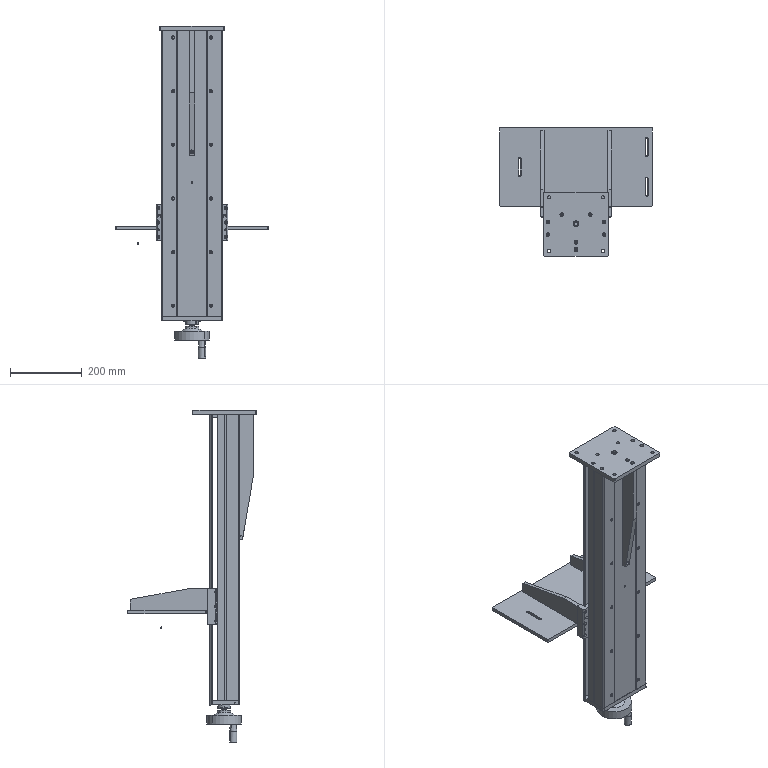Part | STEP file | 170升降-800mm立柱 | 23 solids | 1234 faces | box 425 x 361 x 928 mm | volume 5606632 mm3 | cylinder 592 | plane 372 | cone 154 | sphere 60 | torus 56 | commonest cylinder face diameters 4.2 x104 5.5 x84 9 x76 10 x42 5 x38 6 x30